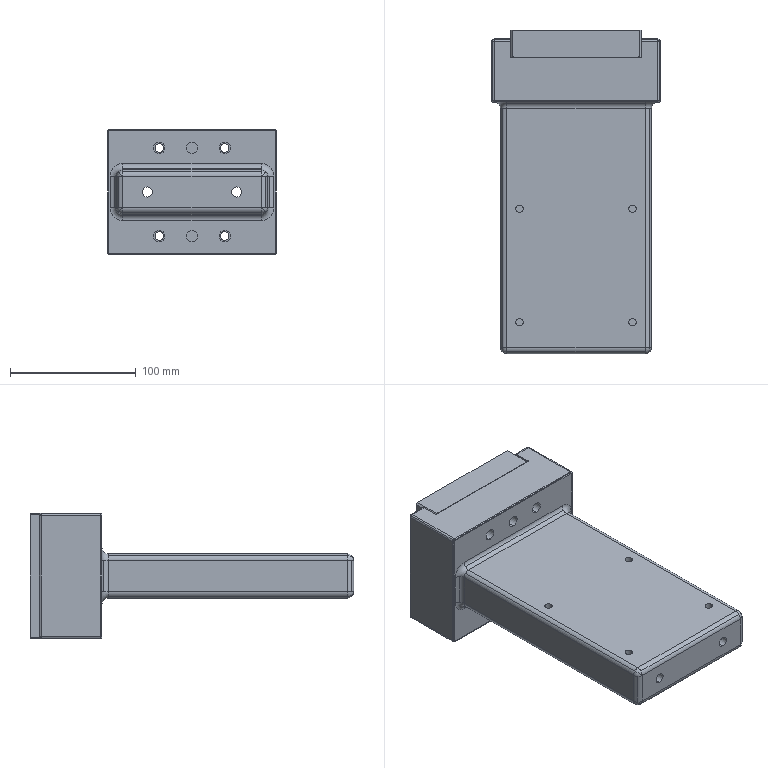Part | STEP file | Sopote_cabina | 2 solids | 153 faces | box 134.1 x 257 x 100 mm | volume 1531756 mm3 | cylinder 92 | plane 35 | sphere 14 | cone 4 | spline 4 | torus 4 | commonest cylinder face diameters 10 x24 4 x18 9 x12 2 x8 6 x8 6.8 x8